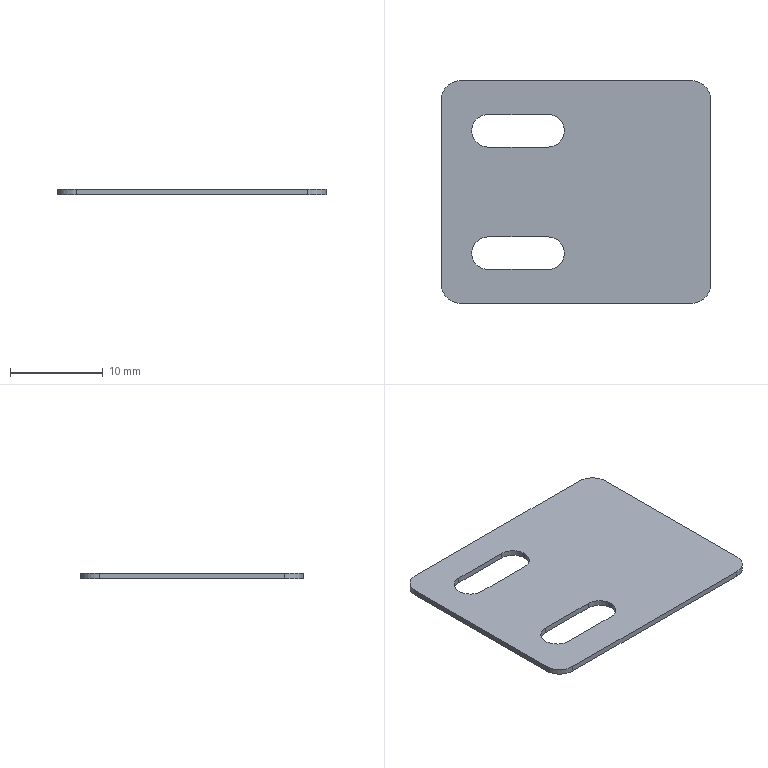Part | STEP file | 10000020545swp000-1 | 1 solid | 20 faces | box 29 x 24 x 0.6 mm | volume 376.694 mm3 | cylinder 10 | plane 10 | commonest cylinder face diameters 3.5 x6 4 x4
STEP:
#1=CARTESIAN_POINT('',(-1.25,-6.6,0.));
#2=VERTEX_POINT('',#1);
#3=CARTESIAN_POINT('',(-3.,-4.85,0.));
#4=VERTEX_POINT('',#3);
#5=CARTESIAN_POINT('',(-3.,-6.6,0.));
#6=DIRECTION('',(0.,0.,1.));
#7=DIRECTION('',(-1.,0.,0.));
#8=AXIS2_PLACEMENT_3D('',#5,#6,#7);
#9=CIRCLE('',#8,1.75);
#10=EDGE_CURVE('',#2,#4,#9,.T.);
#11=ORIENTED_EDGE('',*,*,#10,.F.);
#12=CARTESIAN_POINT('',(-1.25,-6.6,0.6));
#13=VERTEX_POINT('',#12);
#14=CARTESIAN_POINT('',(-1.25,-6.6,0.));
#15=DIRECTION('',(0.,0.,1.));
#16=VECTOR('',#15,1000.);
#17=LINE('',#14,#16);
#18=EDGE_CURVE('',#2,#13,#17,.T.);
#19=ORIENTED_EDGE('',*,*,#18,.T.);
#20=CARTESIAN_POINT('',(-3.,-4.85,0.6));
#21=VERTEX_POINT('',#20);
#22=CARTESIAN_POINT('',(-3.,-6.6,0.6));
#23=DIRECTION('',(0.,0.,1.));
#24=DIRECTION('',(-1.,0.,0.));
#25=AXIS2_PLACEMENT_3D('',#22,#23,#24);
#26=CIRCLE('',#25,1.75);
#27=EDGE_CURVE('',#13,#21,#26,.T.);
#28=ORIENTED_EDGE('',*,*,#27,.T.);
#29=CARTESIAN_POINT('',(-3.,-4.85,0.));
#30=DIRECTION('',(0.,0.,1.));
#31=VECTOR('',#30,1000.);
#32=LINE('',#29,#31);
#33=EDGE_CURVE('',#4,#21,#32,.T.);
#34=ORIENTED_EDGE('',*,*,#33,.F.);
#35=EDGE_LOOP('',(#11,#19,#28,#34));
#36=FACE_OUTER_BOUND('',#35,.T.);
#37=CARTESIAN_POINT('',(-3.,-6.6,0.));
#38=DIRECTION('',(0.,0.,1.));
#39=DIRECTION('',(1.,0.,0.));
#40=AXIS2_PLACEMENT_3D('',#37,#38,#39);
#41=CYLINDRICAL_SURFACE('',#40,1.75);
#42=ADVANCED_FACE('',(#36),#41,.F.);
#43=CARTESIAN_POINT('',(-1.25,6.6,0.));
#44=VERTEX_POINT('',#43);
#45=CARTESIAN_POINT('',(-3.,8.35,0.));
#46=VERTEX_POINT('',#45);
#47=CARTESIAN_POINT('',(-3.,6.6,0.));
#48=DIRECTION('',(0.,0.,1.));
#49=DIRECTION('',(1.,0.,0.));
#50=AXIS2_PLACEMENT_3D('',#47,#48,#49);
#51=CIRCLE('',#50,1.75);
#52=EDGE_CURVE('',#44,#46,#51,.T.);
#53=ORIENTED_EDGE('',*,*,#52,.F.);
#54=CARTESIAN_POINT('',(-1.25,6.6,0.6));
#55=VERTEX_POINT('',#54);
#56=CARTESIAN_POINT('',(-1.25,6.6,0.));
#57=DIRECTION('',(0.,0.,1.));
#58=VECTOR('',#57,1000.);
#59=LINE('',#56,#58);
#60=EDGE_CURVE('',#44,#55,#59,.T.);
#61=ORIENTED_EDGE('',*,*,#60,.T.);
#62=CARTESIAN_POINT('',(-3.,8.35,0.6));
#63=VERTEX_POINT('',#62);
#64=CARTESIAN_POINT('',(-3.,6.6,0.6));
#65=DIRECTION('',(0.,0.,1.));
#66=DIRECTION('',(1.,0.,0.));
#67=AXIS2_PLACEMENT_3D('',#64,#65,#66);
#68=CIRCLE('',#67,1.75);
#69=EDGE_CURVE('',#55,#63,#68,.T.);
#70=ORIENTED_EDGE('',*,*,#69,.T.);
#71=CARTESIAN_POINT('',(-3.,8.35,0.));
#72=DIRECTION('',(0.,0.,1.));
#73=VECTOR('',#72,1000.);
#74=LINE('',#71,#73);
#75=EDGE_CURVE('',#46,#63,#74,.T.);
#76=ORIENTED_EDGE('',*,*,#75,.F.);
#77=EDGE_LOOP('',(#53,#61,#70,#76));
#78=FACE_OUTER_BOUND('',#77,.T.);
#79=CARTESIAN_POINT('',(-3.,6.6,0.));
#80=DIRECTION('',(0.,0.,1.));
#81=DIRECTION('',(1.,0.,0.));
#82=AXIS2_PLACEMENT_3D('',#79,#80,#81);
#83=CYLINDRICAL_SURFACE('',#82,1.75);
#84=ADVANCED_FACE('',(#78),#83,.F.);
#85=CARTESIAN_POINT('',(-14.5,-10.,0.));
#86=VERTEX_POINT('',#85);
#87=CARTESIAN_POINT('',(-12.5,-12.,0.));
#88=VERTEX_POINT('',#87);
#89=CARTESIAN_POINT('',(-12.5,-10.,0.));
#90=DIRECTION('',(0.,0.,1.));
#91=DIRECTION('',(1.,0.,0.));
#92=AXIS2_PLACEMENT_3D('',#89,#90,#91);
#93=CIRCLE('',#92,2.);
#94=EDGE_CURVE('',#86,#88,#93,.T.);
#95=ORIENTED_EDGE('',*,*,#94,.T.);
#96=CARTESIAN_POINT('',(-12.5,-12.,0.6));
#97=VERTEX_POINT('',#96);
#98=CARTESIAN_POINT('',(-12.5,-12.,0.6));
#99=DIRECTION('',(0.,0.,-1.));
#100=VECTOR('',#99,1000.);
#101=LINE('',#98,#100);
#102=EDGE_CURVE('',#97,#88,#101,.T.);
#103=ORIENTED_EDGE('',*,*,#102,.F.);
#104=CARTESIAN_POINT('',(-14.5,-10.,0.6));
#105=VERTEX_POINT('',#104);
#106=CARTESIAN_POINT('',(-12.5,-10.,0.6));
#107=DIRECTION('',(0.,0.,1.));
#108=DIRECTION('',(1.,0.,0.));
#109=AXIS2_PLACEMENT_3D('',#106,#107,#108);
#110=CIRCLE('',#109,2.);
#111=EDGE_CURVE('',#105,#97,#110,.T.);
#112=ORIENTED_EDGE('',*,*,#111,.F.);
#113=CARTESIAN_POINT('',(-14.5,-10.,0.6));
#114=DIRECTION('',(0.,0.,-1.));
#115=VECTOR('',#114,1000.);
#116=LINE('',#113,#115);
#117=EDGE_CURVE('',#105,#86,#116,.T.);
#118=ORIENTED_EDGE('',*,*,#117,.T.);
#119=EDGE_LOOP('',(#95,#103,#112,#118));
#120=FACE_OUTER_BOUND('',#119,.T.);
#121=CARTESIAN_POINT('',(-12.5,-10.,0.6));
#122=DIRECTION('',(0.,0.,-1.));
#123=DIRECTION('',(-1.,0.,0.));
#124=AXIS2_PLACEMENT_3D('',#121,#122,#123);
#125=CYLINDRICAL_SURFACE('',#124,2.);
#126=ADVANCED_FACE('',(#120),#125,.T.);
#127=CARTESIAN_POINT('',(12.5,-12.,0.));
#128=VERTEX_POINT('',#127);
#129=CARTESIAN_POINT('',(-12.5,-12.,0.));
#130=DIRECTION('',(1.,0.,0.));
#131=VECTOR('',#130,1000.);
#132=LINE('',#129,#131);
#133=EDGE_CURVE('',#88,#128,#132,.T.);
#134=ORIENTED_EDGE('',*,*,#133,.T.);
#135=CARTESIAN_POINT('',(12.5,-12.,0.6));
#136=VERTEX_POINT('',#135);
#137=CARTESIAN_POINT('',(12.5,-12.,0.6));
#138=DIRECTION('',(0.,0.,-1.));
#139=VECTOR('',#138,1000.);
#140=LINE('',#137,#139);
#141=EDGE_CURVE('',#136,#128,#140,.T.);
#142=ORIENTED_EDGE('',*,*,#141,.F.);
#143=CARTESIAN_POINT('',(-12.5,-12.,0.6));
#144=DIRECTION('',(1.,0.,0.));
#145=VECTOR('',#144,1000.);
#146=LINE('',#143,#145);
#147=EDGE_CURVE('',#97,#136,#146,.T.);
#148=ORIENTED_EDGE('',*,*,#147,.F.);
#149=ORIENTED_EDGE('',*,*,#102,.T.);
#150=EDGE_LOOP('',(#134,#142,#148,#149));
#151=FACE_OUTER_BOUND('',#150,.T.);
#152=CARTESIAN_POINT('',(-12.5,-12.,0.6));
#153=DIRECTION('',(0.,1.,0.));
#154=DIRECTION('',(0.,0.,1.));
#155=AXIS2_PLACEMENT_3D('',#152,#153,#154);
#156=PLANE('',#155);
#157=ADVANCED_FACE('',(#151),#156,.F.);
#158=CARTESIAN_POINT('',(14.5,-10.,0.));
#159=VERTEX_POINT('',#158);
#160=CARTESIAN_POINT('',(12.5,-10.,0.));
#161=DIRECTION('',(0.,0.,1.));
#162=DIRECTION('',(1.,0.,0.));
#163=AXIS2_PLACEMENT_3D('',#160,#161,#162);
#164=CIRCLE('',#163,2.);
#165=EDGE_CURVE('',#128,#159,#164,.T.);
#166=ORIENTED_EDGE('',*,*,#165,.T.);
#167=CARTESIAN_POINT('',(14.5,-10.,0.6));
#168=VERTEX_POINT('',#167);
#169=CARTESIAN_POINT('',(14.5,-10.,0.6));
#170=DIRECTION('',(0.,0.,-1.));
#171=VECTOR('',#170,1000.);
#172=LINE('',#169,#171);
#173=EDGE_CURVE('',#168,#159,#172,.T.);
#174=ORIENTED_EDGE('',*,*,#173,.F.);
#175=CARTESIAN_POINT('',(12.5,-10.,0.6));
#176=DIRECTION('',(0.,0.,1.));
#177=DIRECTION('',(1.,0.,0.));
#178=AXIS2_PLACEMENT_3D('',#175,#176,#177);
#179=CIRCLE('',#178,2.);
#180=EDGE_CURVE('',#136,#168,#179,.T.);
#181=ORIENTED_EDGE('',*,*,#180,.F.);
#182=ORIENTED_EDGE('',*,*,#141,.T.);
#183=EDGE_LOOP('',(#166,#174,#181,#182));
#184=FACE_OUTER_BOUND('',#183,.T.);
#185=CARTESIAN_POINT('',(12.5,-10.,0.6));
#186=DIRECTION('',(0.,0.,-1.));
#187=DIRECTION('',(-1.,0.,0.));
#188=AXIS2_PLACEMENT_3D('',#185,#186,#187);
#189=CYLINDRICAL_SURFACE('',#188,2.);
#190=ADVANCED_FACE('',(#184),#189,.T.);
#191=CARTESIAN_POINT('',(14.5,10.,0.));
#192=VERTEX_POINT('',#191);
#193=CARTESIAN_POINT('',(14.5,-10.,0.));
#194=DIRECTION('',(0.,1.,0.));
#195=VECTOR('',#194,1000.);
#196=LINE('',#193,#195);
#197=EDGE_CURVE('',#159,#192,#196,.T.);
#198=ORIENTED_EDGE('',*,*,#197,.T.);
#199=CARTESIAN_POINT('',(14.5,10.,0.6));
#200=VERTEX_POINT('',#199);
#201=CARTESIAN_POINT('',(14.5,10.,0.6));
#202=DIRECTION('',(0.,0.,-1.));
#203=VECTOR('',#202,1000.);
#204=LINE('',#201,#203);
#205=EDGE_CURVE('',#200,#192,#204,.T.);
#206=ORIENTED_EDGE('',*,*,#205,.F.);
#207=CARTESIAN_POINT('',(14.5,-10.,0.6));
#208=DIRECTION('',(0.,1.,0.));
#209=VECTOR('',#208,1000.);
#210=LINE('',#207,#209);
#211=EDGE_CURVE('',#168,#200,#210,.T.);
#212=ORIENTED_EDGE('',*,*,#211,.F.);
#213=ORIENTED_EDGE('',*,*,#173,.T.);
#214=EDGE_LOOP('',(#198,#206,#212,#213));
#215=FACE_OUTER_BOUND('',#214,.T.);
#216=CARTESIAN_POINT('',(14.5,-10.,0.6));
#217=DIRECTION('',(-1.,0.,0.));
#218=DIRECTION('',(0.,0.,1.));
#219=AXIS2_PLACEMENT_3D('',#216,#217,#218);
#220=PLANE('',#219);
#221=ADVANCED_FACE('',(#215),#220,.F.);
#222=CARTESIAN_POINT('',(12.5,12.,0.));
#223=VERTEX_POINT('',#222);
#224=CARTESIAN_POINT('',(12.5,10.,0.));
#225=DIRECTION('',(0.,0.,1.));
#226=DIRECTION('',(-1.,0.,0.));
#227=AXIS2_PLACEMENT_3D('',#224,#225,#226);
#228=CIRCLE('',#227,2.);
#229=EDGE_CURVE('',#192,#223,#228,.T.);
#230=ORIENTED_EDGE('',*,*,#229,.T.);
#231=CARTESIAN_POINT('',(12.5,12.,0.6));
#232=VERTEX_POINT('',#231);
#233=CARTESIAN_POINT('',(12.5,12.,0.6));
#234=DIRECTION('',(0.,0.,-1.));
#235=VECTOR('',#234,1000.);
#236=LINE('',#233,#235);
#237=EDGE_CURVE('',#232,#223,#236,.T.);
#238=ORIENTED_EDGE('',*,*,#237,.F.);
#239=CARTESIAN_POINT('',(12.5,10.,0.6));
#240=DIRECTION('',(0.,0.,1.));
#241=DIRECTION('',(-1.,0.,0.));
#242=AXIS2_PLACEMENT_3D('',#239,#240,#241);
#243=CIRCLE('',#242,2.);
#244=EDGE_CURVE('',#200,#232,#243,.T.);
#245=ORIENTED_EDGE('',*,*,#244,.F.);
#246=ORIENTED_EDGE('',*,*,#205,.T.);
#247=EDGE_LOOP('',(#230,#238,#245,#246));
#248=FACE_OUTER_BOUND('',#247,.T.);
#249=CARTESIAN_POINT('',(12.5,10.,0.6));
#250=DIRECTION('',(0.,0.,-1.));
#251=DIRECTION('',(-1.,0.,0.));
#252=AXIS2_PLACEMENT_3D('',#249,#250,#251);
#253=CYLINDRICAL_SURFACE('',#252,2.);
#254=ADVANCED_FACE('',(#248),#253,.T.);
#255=CARTESIAN_POINT('',(-12.5,12.,0.));
#256=VERTEX_POINT('',#255);
#257=CARTESIAN_POINT('',(-12.5,12.,0.));
#258=DIRECTION('',(-1.,0.,0.));
#259=VECTOR('',#258,1000.);
#260=LINE('',#257,#259);
#261=EDGE_CURVE('',#223,#256,#260,.T.);
#262=ORIENTED_EDGE('',*,*,#261,.T.);
#263=CARTESIAN_POINT('',(-12.5,12.,0.6));
#264=VERTEX_POINT('',#263);
#265=CARTESIAN_POINT('',(-12.5,12.,0.6));
#266=DIRECTION('',(0.,0.,-1.));
#267=VECTOR('',#266,1000.);
#268=LINE('',#265,#267);
#269=EDGE_CURVE('',#264,#256,#268,.T.);
#270=ORIENTED_EDGE('',*,*,#269,.F.);
#271=CARTESIAN_POINT('',(-12.5,12.,0.6));
#272=DIRECTION('',(-1.,0.,0.));
#273=VECTOR('',#272,1000.);
#274=LINE('',#271,#273);
#275=EDGE_CURVE('',#232,#264,#274,.T.);
#276=ORIENTED_EDGE('',*,*,#275,.F.);
#277=ORIENTED_EDGE('',*,*,#237,.T.);
#278=EDGE_LOOP('',(#262,#270,#276,#277));
#279=FACE_OUTER_BOUND('',#278,.T.);
#280=CARTESIAN_POINT('',(-12.5,12.,0.6));
#281=DIRECTION('',(0.,-1.,0.));
#282=DIRECTION('',(0.,0.,-1.));
#283=AXIS2_PLACEMENT_3D('',#280,#281,#282);
#284=PLANE('',#283);
#285=ADVANCED_FACE('',(#279),#284,.F.);
#286=CARTESIAN_POINT('',(-14.5,10.,0.));
#287=VERTEX_POINT('',#286);
#288=CARTESIAN_POINT('',(-12.5,10.,0.));
#289=DIRECTION('',(0.,0.,1.));
#290=DIRECTION('',(1.,0.,0.));
#291=AXIS2_PLACEMENT_3D('',#288,#289,#290);
#292=CIRCLE('',#291,2.);
#293=EDGE_CURVE('',#256,#287,#292,.T.);
#294=ORIENTED_EDGE('',*,*,#293,.T.);
#295=CARTESIAN_POINT('',(-14.5,10.,0.6));
#296=VERTEX_POINT('',#295);
#297=CARTESIAN_POINT('',(-14.5,10.,0.6));
#298=DIRECTION('',(0.,0.,-1.));
#299=VECTOR('',#298,1000.);
#300=LINE('',#297,#299);
#301=EDGE_CURVE('',#296,#287,#300,.T.);
#302=ORIENTED_EDGE('',*,*,#301,.F.);
#303=CARTESIAN_POINT('',(-12.5,10.,0.6));
#304=DIRECTION('',(0.,0.,1.));
#305=DIRECTION('',(1.,0.,0.));
#306=AXIS2_PLACEMENT_3D('',#303,#304,#305);
#307=CIRCLE('',#306,2.);
#308=EDGE_CURVE('',#264,#296,#307,.T.);
#309=ORIENTED_EDGE('',*,*,#308,.F.);
#310=ORIENTED_EDGE('',*,*,#269,.T.);
#311=EDGE_LOOP('',(#294,#302,#309,#310));
#312=FACE_OUTER_BOUND('',#311,.T.);
#313=CARTESIAN_POINT('',(-12.5,10.,0.6));
#314=DIRECTION('',(0.,0.,-1.));
#315=DIRECTION('',(-1.,0.,0.));
#316=AXIS2_PLACEMENT_3D('',#313,#314,#315);
#317=CYLINDRICAL_SURFACE('',#316,2.);
#318=ADVANCED_FACE('',(#312),#317,.T.);
#319=CARTESIAN_POINT('',(-14.5,-10.,0.));
#320=DIRECTION('',(0.,-1.,0.));
#321=VECTOR('',#320,1000.);
#322=LINE('',#319,#321);
#323=EDGE_CURVE('',#287,#86,#322,.T.);
#324=ORIENTED_EDGE('',*,*,#323,.T.);
#325=ORIENTED_EDGE('',*,*,#117,.F.);
#326=CARTESIAN_POINT('',(-14.5,-10.,0.6));
#327=DIRECTION('',(0.,-1.,0.));
#328=VECTOR('',#327,1000.);
#329=LINE('',#326,#328);
#330=EDGE_CURVE('',#296,#105,#329,.T.);
#331=ORIENTED_EDGE('',*,*,#330,.F.);
#332=ORIENTED_EDGE('',*,*,#301,.T.);
#333=EDGE_LOOP('',(#324,#325,#331,#332));
#334=FACE_OUTER_BOUND('',#333,.T.);
#335=CARTESIAN_POINT('',(-14.5,-10.,0.6));
#336=DIRECTION('',(1.,0.,0.));
#337=DIRECTION('',(0.,0.,-1.));
#338=AXIS2_PLACEMENT_3D('',#335,#336,#337);
#339=PLANE('',#338);
#340=ADVANCED_FACE('',(#334),#339,.F.);
#341=CARTESIAN_POINT('',(-9.5,-4.85,0.6));
#342=VERTEX_POINT('',#341);
#343=CARTESIAN_POINT('',(-9.5,-8.35,0.6));
#344=VERTEX_POINT('',#343);
#345=CARTESIAN_POINT('',(-9.5,-6.6,0.6));
#346=DIRECTION('',(0.,0.,1.));
#347=DIRECTION('',(-1.,0.,0.));
#348=AXIS2_PLACEMENT_3D('',#345,#346,#347);
#349=CIRCLE('',#348,1.75);
#350=EDGE_CURVE('',#342,#344,#349,.T.);
#351=ORIENTED_EDGE('',*,*,#350,.F.);
#352=CARTESIAN_POINT('',(-9.5,-4.85,0.6));
#353=DIRECTION('',(-1.,0.,0.));
#354=VECTOR('',#353,1000.);
#355=LINE('',#352,#354);
#356=EDGE_CURVE('',#21,#342,#355,.T.);
#357=ORIENTED_EDGE('',*,*,#356,.F.);
#358=ORIENTED_EDGE('',*,*,#27,.F.);
#359=CARTESIAN_POINT('',(-3.,-8.35,0.6));
#360=VERTEX_POINT('',#359);
#361=CARTESIAN_POINT('',(-3.,-6.6,0.6));
#362=DIRECTION('',(0.,0.,1.));
#363=DIRECTION('',(-1.,0.,0.));
#364=AXIS2_PLACEMENT_3D('',#361,#362,#363);
#365=CIRCLE('',#364,1.75);
#366=EDGE_CURVE('',#360,#13,#365,.T.);
#367=ORIENTED_EDGE('',*,*,#366,.F.);
#368=CARTESIAN_POINT('',(-9.5,-8.35,0.6));
#369=DIRECTION('',(1.,0.,0.));
#370=VECTOR('',#369,1000.);
#371=LINE('',#368,#370);
#372=EDGE_CURVE('',#344,#360,#371,.T.);
#373=ORIENTED_EDGE('',*,*,#372,.F.);
#374=EDGE_LOOP('',(#351,#357,#358,#367,#373));
#375=FACE_BOUND('',#374,.T.);
#376=CARTESIAN_POINT('',(-9.5,8.35,0.6));
#377=VERTEX_POINT('',#376);
#378=CARTESIAN_POINT('',(-9.5,4.85,0.6));
#379=VERTEX_POINT('',#378);
#380=CARTESIAN_POINT('',(-9.5,6.6,0.6));
#381=DIRECTION('',(0.,0.,1.));
#382=DIRECTION('',(1.,0.,0.));
#383=AXIS2_PLACEMENT_3D('',#380,#381,#382);
#384=CIRCLE('',#383,1.75);
#385=EDGE_CURVE('',#377,#379,#384,.T.);
#386=ORIENTED_EDGE('',*,*,#385,.F.);
#387=CARTESIAN_POINT('',(-9.5,8.35,0.6));
#388=DIRECTION('',(-1.,0.,0.));
#389=VECTOR('',#388,1000.);
#390=LINE('',#387,#389);
#391=EDGE_CURVE('',#63,#377,#390,.T.);
#392=ORIENTED_EDGE('',*,*,#391,.F.);
#393=ORIENTED_EDGE('',*,*,#69,.F.);
#394=CARTESIAN_POINT('',(-3.,4.85,0.6));
#395=VERTEX_POINT('',#394);
#396=CARTESIAN_POINT('',(-3.,6.6,0.6));
#397=DIRECTION('',(0.,0.,1.));
#398=DIRECTION('',(1.,0.,0.));
#399=AXIS2_PLACEMENT_3D('',#396,#397,#398);
#400=CIRCLE('',#399,1.75);
#401=EDGE_CURVE('',#395,#55,#400,.T.);
#402=ORIENTED_EDGE('',*,*,#401,.F.);
#403=CARTESIAN_POINT('',(-9.5,4.85,0.6));
#404=DIRECTION('',(1.,0.,0.));
#405=VECTOR('',#404,1000.);
#406=LINE('',#403,#405);
#407=EDGE_CURVE('',#379,#395,#406,.T.);
#408=ORIENTED_EDGE('',*,*,#407,.F.);
#409=EDGE_LOOP('',(#386,#392,#393,#402,#408));
#410=FACE_BOUND('',#409,.T.);
#411=ORIENTED_EDGE('',*,*,#111,.T.);
#412=ORIENTED_EDGE('',*,*,#147,.T.);
#413=ORIENTED_EDGE('',*,*,#180,.T.);
#414=ORIENTED_EDGE('',*,*,#211,.T.);
#415=ORIENTED_EDGE('',*,*,#244,.T.);
#416=ORIENTED_EDGE('',*,*,#275,.T.);
#417=ORIENTED_EDGE('',*,*,#308,.T.);
#418=ORIENTED_EDGE('',*,*,#330,.T.);
#419=EDGE_LOOP('',(#411,#412,#413,#414,#415,#416,#417,#418));
#420=FACE_OUTER_BOUND('',#419,.T.);
#421=CARTESIAN_POINT('',(-12.5,-10.,0.6));
#422=DIRECTION('',(0.,0.,1.));
#423=DIRECTION('',(1.,0.,0.));
#424=AXIS2_PLACEMENT_3D('',#421,#422,#423);
#425=PLANE('',#424);
#426=ADVANCED_FACE('',(#375,#410,#420),#425,.T.);
#427=CARTESIAN_POINT('',(-9.5,-4.85,0.));
#428=VERTEX_POINT('',#427);
#429=CARTESIAN_POINT('',(-9.5,-4.85,0.));
#430=DIRECTION('',(-1.,0.,0.));
#431=VECTOR('',#430,1000.);
#432=LINE('',#429,#431);
#433=EDGE_CURVE('',#4,#428,#432,.T.);
#434=ORIENTED_EDGE('',*,*,#433,.T.);
#435=CARTESIAN_POINT('',(-9.5,-8.35,0.));
#436=VERTEX_POINT('',#435);
#437=CARTESIAN_POINT('',(-9.5,-6.6,0.));
#438=DIRECTION('',(0.,0.,1.));
#439=DIRECTION('',(-1.,0.,0.));
#440=AXIS2_PLACEMENT_3D('',#437,#438,#439);
#441=CIRCLE('',#440,1.75);
#442=EDGE_CURVE('',#428,#436,#441,.T.);
#443=ORIENTED_EDGE('',*,*,#442,.T.);
#444=CARTESIAN_POINT('',(-3.,-8.35,0.));
#445=VERTEX_POINT('',#444);
#446=CARTESIAN_POINT('',(-9.5,-8.35,0.));
#447=DIRECTION('',(1.,0.,0.));
#448=VECTOR('',#447,1000.);
#449=LINE('',#446,#448);
#450=EDGE_CURVE('',#436,#445,#449,.T.);
#451=ORIENTED_EDGE('',*,*,#450,.T.);
#452=CARTESIAN_POINT('',(-3.,-6.6,0.));
#453=DIRECTION('',(0.,0.,1.));
#454=DIRECTION('',(-1.,0.,0.));
#455=AXIS2_PLACEMENT_3D('',#452,#453,#454);
#456=CIRCLE('',#455,1.75);
#457=EDGE_CURVE('',#445,#2,#456,.T.);
#458=ORIENTED_EDGE('',*,*,#457,.T.);
#459=ORIENTED_EDGE('',*,*,#10,.T.);
#460=EDGE_LOOP('',(#434,#443,#451,#458,#459));
#461=FACE_BOUND('',#460,.T.);
#462=CARTESIAN_POINT('',(-9.5,8.35,0.));
#463=VERTEX_POINT('',#462);
#464=CARTESIAN_POINT('',(-9.5,8.35,0.));
#465=DIRECTION('',(-1.,0.,0.));
#466=VECTOR('',#465,1000.);
#467=LINE('',#464,#466);
#468=EDGE_CURVE('',#46,#463,#467,.T.);
#469=ORIENTED_EDGE('',*,*,#468,.T.);
#470=CARTESIAN_POINT('',(-9.5,4.85,0.));
#471=VERTEX_POINT('',#470);
#472=CARTESIAN_POINT('',(-9.5,6.6,0.));
#473=DIRECTION('',(0.,0.,1.));
#474=DIRECTION('',(1.,0.,0.));
#475=AXIS2_PLACEMENT_3D('',#472,#473,#474);
#476=CIRCLE('',#475,1.75);
#477=EDGE_CURVE('',#463,#471,#476,.T.);
#478=ORIENTED_EDGE('',*,*,#477,.T.);
#479=CARTESIAN_POINT('',(-3.,4.85,0.));
#480=VERTEX_POINT('',#479);
#481=CARTESIAN_POINT('',(-9.5,4.85,0.));
#482=DIRECTION('',(1.,0.,0.));
#483=VECTOR('',#482,1000.);
#484=LINE('',#481,#483);
#485=EDGE_CURVE('',#471,#480,#484,.T.);
#486=ORIENTED_EDGE('',*,*,#485,.T.);
#487=CARTESIAN_POINT('',(-3.,6.6,0.));
#488=DIRECTION('',(0.,0.,1.));
#489=DIRECTION('',(1.,0.,0.));
#490=AXIS2_PLACEMENT_3D('',#487,#488,#489);
#491=CIRCLE('',#490,1.75);
#492=EDGE_CURVE('',#480,#44,#491,.T.);
#493=ORIENTED_EDGE('',*,*,#492,.T.);
#494=ORIENTED_EDGE('',*,*,#52,.T.);
#495=EDGE_LOOP('',(#469,#478,#486,#493,#494));
#496=FACE_BOUND('',#495,.T.);
#497=ORIENTED_EDGE('',*,*,#94,.F.);
#498=ORIENTED_EDGE('',*,*,#323,.F.);
#499=ORIENTED_EDGE('',*,*,#293,.F.);
#500=ORIENTED_EDGE('',*,*,#261,.F.);
#501=ORIENTED_EDGE('',*,*,#229,.F.);
#502=ORIENTED_EDGE('',*,*,#197,.F.);
#503=ORIENTED_EDGE('',*,*,#165,.F.);
#504=ORIENTED_EDGE('',*,*,#133,.F.);
#505=EDGE_LOOP('',(#497,#498,#499,#500,#501,#502,#503,#504));
#506=FACE_OUTER_BOUND('',#505,.T.);
#507=CARTESIAN_POINT('',(-12.5,-10.,0.));
#508=DIRECTION('',(0.,0.,1.));
#509=DIRECTION('',(1.,0.,0.));
#510=AXIS2_PLACEMENT_3D('',#507,#508,#509);
#511=PLANE('',#510);
#512=ADVANCED_FACE('',(#461,#496,#506),#511,.F.);
#513=ORIENTED_EDGE('',*,*,#385,.T.);
#514=CARTESIAN_POINT('',(-9.5,4.85,0.));
#515=DIRECTION('',(0.,0.,1.));
#516=VECTOR('',#515,1000.);
#517=LINE('',#514,#516);
#518=EDGE_CURVE('',#471,#379,#517,.T.);
#519=ORIENTED_EDGE('',*,*,#518,.F.);
#520=ORIENTED_EDGE('',*,*,#477,.F.);
#521=CARTESIAN_POINT('',(-9.5,8.35,0.));
#522=DIRECTION('',(0.,0.,1.));
#523=VECTOR('',#522,1000.);
#524=LINE('',#521,#523);
#525=EDGE_CURVE('',#463,#377,#524,.T.);
#526=ORIENTED_EDGE('',*,*,#525,.T.);
#527=EDGE_LOOP('',(#513,#519,#520,#526));
#528=FACE_OUTER_BOUND('',#527,.T.);
#529=CARTESIAN_POINT('',(-9.5,6.6,0.));
#530=DIRECTION('',(0.,0.,1.));
#531=DIRECTION('',(1.,0.,0.));
#532=AXIS2_PLACEMENT_3D('',#529,#530,#531);
#533=CYLINDRICAL_SURFACE('',#532,1.75);
#534=ADVANCED_FACE('',(#528),#533,.F.);
#535=ORIENTED_EDGE('',*,*,#391,.T.);
#536=ORIENTED_EDGE('',*,*,#525,.F.);
#537=ORIENTED_EDGE('',*,*,#468,.F.);
#538=ORIENTED_EDGE('',*,*,#75,.T.);
#539=EDGE_LOOP('',(#535,#536,#537,#538));
#540=FACE_OUTER_BOUND('',#539,.T.);
#541=CARTESIAN_POINT('',(-9.5,8.35,0.));
#542=DIRECTION('',(0.,1.,0.));
#543=DIRECTION('',(0.,0.,1.));
#544=AXIS2_PLACEMENT_3D('',#541,#542,#543);
#545=PLANE('',#544);
#546=ADVANCED_FACE('',(#540),#545,.F.);
#547=ORIENTED_EDGE('',*,*,#60,.F.);
#548=ORIENTED_EDGE('',*,*,#492,.F.);
#549=CARTESIAN_POINT('',(-3.,4.85,0.));
#550=DIRECTION('',(0.,0.,1.));
#551=VECTOR('',#550,1000.);
#552=LINE('',#549,#551);
#553=EDGE_CURVE('',#480,#395,#552,.T.);
#554=ORIENTED_EDGE('',*,*,#553,.T.);
#555=ORIENTED_EDGE('',*,*,#401,.T.);
#556=EDGE_LOOP('',(#547,#548,#554,#555));
#557=FACE_OUTER_BOUND('',#556,.T.);
#558=CARTESIAN_POINT('',(-3.,6.6,0.));
#559=DIRECTION('',(0.,0.,1.));
#560=DIRECTION('',(1.,0.,0.));
#561=AXIS2_PLACEMENT_3D('',#558,#559,#560);
#562=CYLINDRICAL_SURFACE('',#561,1.75);
#563=ADVANCED_FACE('',(#557),#562,.F.);
#564=ORIENTED_EDGE('',*,*,#407,.T.);
#565=ORIENTED_EDGE('',*,*,#553,.F.);
#566=ORIENTED_EDGE('',*,*,#485,.F.);
#567=ORIENTED_EDGE('',*,*,#518,.T.);
#568=EDGE_LOOP('',(#564,#565,#566,#567));
#569=FACE_OUTER_BOUND('',#568,.T.);
#570=CARTESIAN_POINT('',(-9.5,4.85,0.));
#571=DIRECTION('',(0.,-1.,0.));
#572=DIRECTION('',(0.,0.,-1.));
#573=AXIS2_PLACEMENT_3D('',#570,#571,#572);
#574=PLANE('',#573);
#575=ADVANCED_FACE('',(#569),#574,.F.);
#576=ORIENTED_EDGE('',*,*,#350,.T.);
#577=CARTESIAN_POINT('',(-9.5,-8.35,0.));
#578=DIRECTION('',(0.,0.,1.));
#579=VECTOR('',#578,1000.);
#580=LINE('',#577,#579);
#581=EDGE_CURVE('',#436,#344,#580,.T.);
#582=ORIENTED_EDGE('',*,*,#581,.F.);
#583=ORIENTED_EDGE('',*,*,#442,.F.);
#584=CARTESIAN_POINT('',(-9.5,-4.85,0.));
#585=DIRECTION('',(0.,0.,1.));
#586=VECTOR('',#585,1000.);
#587=LINE('',#584,#586);
#588=EDGE_CURVE('',#428,#342,#587,.T.);
#589=ORIENTED_EDGE('',*,*,#588,.T.);
#590=EDGE_LOOP('',(#576,#582,#583,#589));
#591=FACE_OUTER_BOUND('',#590,.T.);
#592=CARTESIAN_POINT('',(-9.5,-6.6,0.));
#593=DIRECTION('',(0.,0.,1.));
#594=DIRECTION('',(1.,0.,0.));
#595=AXIS2_PLACEMENT_3D('',#592,#593,#594);
#596=CYLINDRICAL_SURFACE('',#595,1.75);
#597=ADVANCED_FACE('',(#591),#596,.F.);
#598=ORIENTED_EDGE('',*,*,#356,.T.);
#599=ORIENTED_EDGE('',*,*,#588,.F.);
#600=ORIENTED_EDGE('',*,*,#433,.F.);
#601=ORIENTED_EDGE('',*,*,#33,.T.);
#602=EDGE_LOOP('',(#598,#599,#600,#601));
#603=FACE_OUTER_BOUND('',#602,.T.);
#604=CARTESIAN_POINT('',(-9.5,-4.85,0.));
#605=DIRECTION('',(0.,1.,0.));
#606=DIRECTION('',(0.,0.,1.));
#607=AXIS2_PLACEMENT_3D('',#604,#605,#606);
#608=PLANE('',#607);
#609=ADVANCED_FACE('',(#603),#608,.F.);
#610=ORIENTED_EDGE('',*,*,#18,.F.);
#611=ORIENTED_EDGE('',*,*,#457,.F.);
#612=CARTESIAN_POINT('',(-3.,-8.35,0.));
#613=DIRECTION('',(0.,0.,1.));
#614=VECTOR('',#613,1000.);
#615=LINE('',#612,#614);
#616=EDGE_CURVE('',#445,#360,#615,.T.);
#617=ORIENTED_EDGE('',*,*,#616,.T.);
#618=ORIENTED_EDGE('',*,*,#366,.T.);
#619=EDGE_LOOP('',(#610,#611,#617,#618));
#620=FACE_OUTER_BOUND('',#619,.T.);
#621=CARTESIAN_POINT('',(-3.,-6.6,0.));
#622=DIRECTION('',(0.,0.,1.));
#623=DIRECTION('',(1.,0.,0.));
#624=AXIS2_PLACEMENT_3D('',#621,#622,#623);
#625=CYLINDRICAL_SURFACE('',#624,1.75);
#626=ADVANCED_FACE('',(#620),#625,.F.);
#627=ORIENTED_EDGE('',*,*,#372,.T.);
#628=ORIENTED_EDGE('',*,*,#616,.F.);
#629=ORIENTED_EDGE('',*,*,#450,.F.);
#630=ORIENTED_EDGE('',*,*,#581,.T.);
#631=EDGE_LOOP('',(#627,#628,#629,#630));
#632=FACE_OUTER_BOUND('',#631,.T.);
#633=CARTESIAN_POINT('',(-9.5,-8.35,0.));
#634=DIRECTION('',(0.,-1.,0.));
#635=DIRECTION('',(0.,0.,-1.));
#636=AXIS2_PLACEMENT_3D('',#633,#634,#635);
#637=PLANE('',#636);
#638=ADVANCED_FACE('',(#632),#637,.F.);
#639=CLOSED_SHELL('',(#42,#84,#126,#157,#190,#221,#254,#285,#318,#340,#426,#512,#534,#546,#563,#575,#597,#609,#626,#638));
#640=MANIFOLD_SOLID_BREP('',#639);
#641=CARTESIAN_POINT('',(0.,0.,0.));
#642=DIRECTION('',(0.,0.,1.));
#643=DIRECTION('',(1.,0.,0.));
#644=AXIS2_PLACEMENT_3D('',#641,#642,#643);
#645=(LENGTH_UNIT()NAMED_UNIT(*)SI_UNIT(.MILLI.,.METRE.));
#646=UNCERTAINTY_MEASURE_WITH_UNIT(LENGTH_MEASURE(0.00001),#645,'','');
#647=(NAMED_UNIT(*)PLANE_ANGLE_UNIT()SI_UNIT($,.RADIAN.));
#648=(NAMED_UNIT(*)SI_UNIT($,.STERADIAN.)SOLID_ANGLE_UNIT());
#649=(GEOMETRIC_REPRESENTATION_CONTEXT(3)GLOBAL_UNCERTAINTY_ASSIGNED_CONTEXT((#646))GLOBAL_UNIT_ASSIGNED_CONTEXT((#645,#647,#648))REPRESENTATION_CONTEXT('',''));
#650=ADVANCED_BREP_SHAPE_REPRESENTATION('',(#640,#644),#649);